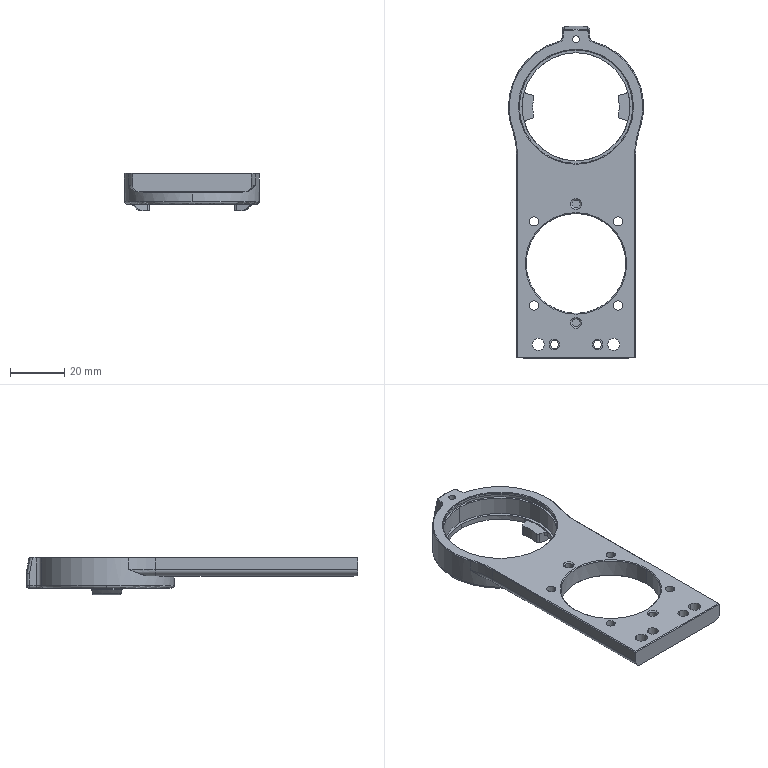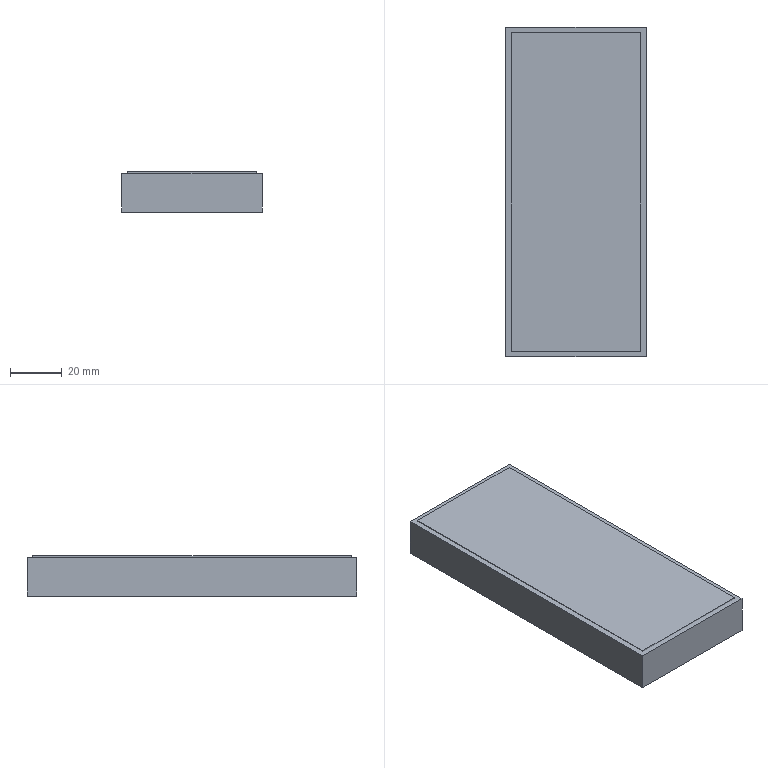CAM job | NX | 3-axis milling, drilling | part box 50 x 122.9 x 14 mm | stock box 54 x 126.9 x 15.5 mm
Tools:
number,name,description,diameter,corner_radius,flute_length,length,flutes
19,D80,Milling Tool-5 Parameters,80.0,0.0,50.0,75.0,2
1,D6A45,Milling Tool-5 Parameters,6.0,0.0,50.0,75.0,2
15,D10,Milling Tool-5 Parameters,10.0,0.0,50.0,75.0,2
14,D10JING,Milling Tool-5 Parameters,10.0,0.0,50.0,75.0,2
8,4.5ZT,Drilling Tool,4.5,0.0,35.0,50.0,2
16,3.0ZT,Drilling Tool,3.0,0.0,35.0,50.0,2
7,3.4ZT,Drilling Tool,3.4,0.0,35.0,50.0,2
2,2.5ZT,Drilling Tool,2.5,0.0,35.0,50.0,2
17,D2,Milling Tool-5 Parameters,2.0,0.0,50.0,75.0,2
18,D3R0.5,Milling Tool-5 Parameters,3.0,0.5,50.0,75.0,2
21,T6H4D1.5,Milling Tool-T Cutter,6.0,,1.5,25.0,4
11,D4,Milling Tool-5 Parameters,4.0,0.0,50.0,75.0,2
Operations:
program,operation,operation_type,tool,method,geometry_group,spindle_rpm,surface_speed,feed_per_tooth,feed_cut,feed_plunge,cut_length_mm,path_length_mm,cut_time_min,machine_time_min
1,FLOOR_WALL,VolumeBased25DMillingOperation,D80,METHOD,A,5000.0,1256.0,0.12,1200.0,100.0,218.9,272.9,0.1824,0.1878
1,ZLEVEL_PROFILE,ZLevelMilling,D10,METHOD,A,9500.0,298.0,0.1842,3500.0,1000.0,6306.798,6377.798,1.833,1.84
1,HOLE_MILLING,CylinderMilling,D10,METHOD,A,9500.0,0.0,0.0,2500.0,1000.0,781.06,847.56,0.3148,0.3214
1,HOLE_MILLING_COPY,CylinderMilling,D10,METHOD,A,9500.0,0.0,0.0,2500.0,1000.0,974.372,1043.872,0.3921,0.3991
1,ZLEVEL_PROFILE_COPY,ZLevelMilling,D10JING,METHOD,A,9500.0,298.0,0.0789,1500.0,1000.0,377.945,462.945,0.2615,0.27
1,HOLE_MILLING_COPY_COPY,CylinderMilling,D10JING,METHOD,A,9500.0,0.0,0.1053,2000.0,1000.0,1146.72,1215.745,0.5829,0.5898
1,HOLE_MILLING_COPY_COPY_COPY,CylinderMilling,D10JING,METHOD,A,9500.0,0.0,0.1053,2000.0,1000.0,287.94,348.44,0.1529,0.159
1,SPOT_DRILLING,Operation,D6A45,METHOD,A,9500.0,179.0,0.0132,250.0,0.0,52.0,415.591,0.208,0.2444
1,DRILLING,Operation,4.5ZT,METHOD,A,2500.0,35.0,0.04,200.0,0.0,18.904,128.968,0.0945,0.1055
1,DRILLING_COPY,Operation,3.0ZT,METHOD,A,2500.0,35.0,0.04,200.0,0.0,24.803,128.884,0.124,0.1344
1,DRILLING_COPY_COPY,Operation,3.4ZT,METHOD,A,2500.0,35.0,0.04,200.0,0.0,50.086,262.943,0.2504,0.2717
1,DRILLING_COPY_COPY_COPY,Operation,2.5ZT,METHOD,A,2500.0,19.0,0.02,100.0,0.0,16.751,93.502,0.1675,0.1752
1,HOLE_MILLING_1,CylinderMilling,D2,METHOD,A,9500.0,59.0,0.0553,1050.0,100.0,639.065,964.378,0.6086,0.6412
1,ZLEVEL_PROFILE_1,ZLevelMilling,D3R0.5,METHOD,A,9500.0,89.0,0.1316,2500.0,1000.0,1324.38,1546.793,0.5389,0.5611
1,ZLEVEL_PROFILE_COPY_1,ZLevelMilling,D3R0.5,METHOD,A,9500.0,298.0,0.1842,3500.0,1000.0,345.377,683.941,0.144,0.1779
1,PLANAR_PROFILE,PlanarMilling,D6A45,METHOD,A,9500.0,179.0,0.0789,1500.0,100.0,715.283,1785.284,0.4769,0.5839
1,PLANAR_MILL,PlanarMilling,T6H4D1.5,METHOD,A,9500.0,179.0,0.0329,1250.0,100.0,366.114,425.114,0.2929,0.2988
2,FLOOR_WALL_COPY,VolumeBased25DMillingOperation,D80,METHOD,B,5000.0,1256.0,0.12,1200.0,100.0,437.8,756.9,0.3648,0.3967
2,FLOOR_WALL_COPY_COPY,VolumeBased25DMillingOperation,D80,METHOD,B,5000.0,1256.0,0.12,1200.0,100.0,218.9,272.9,0.1824,0.1878
2,FLOOR_WALL_1,VolumeBased25DMillingOperation,D10,METHOD,B,9500.0,298.0,0.1316,2500.0,1000.0,6466.524,6677.464,2.786,2.807
2,FLOOR_WALL_1_COPY,VolumeBased25DMillingOperation,D10,METHOD,B,9500.0,298.0,0.1316,2500.0,1000.0,1917.348,2034.197,0.855,0.8667
2,ZLEVEL_PROFILE_COPY_2,ZLevelMilling,D10,METHOD,B,9500.0,298.0,0.1053,2000.0,1000.0,461.743,836.252,0.2434,0.2808
2,FLOOR_WALL_1_COPY_1,VolumeBased25DMillingOperation,D4,METHOD,B,9500.0,119.0,0.1053,2000.0,1000.0,4963.452,5168.629,2.844,2.864
2,FLOOR_WALL_1_COPY_1_COPY,VolumeBased25DMillingOperation,D4,METHOD,B,9500.0,119.0,0.1053,2000.0,1000.0,1096.978,1373.241,0.8775,0.9052
2,HOLE_MILLING_2,CylinderMilling,D4,METHOD,B,9500.0,119.0,0.0658,1250.0,100.0,212.223,394.023,0.1698,0.188
2,FLOOR_WALL_1_COPY_1_COPY_COPY,VolumeBased25DMillingOperation,D4,METHOD,B,9500.0,119.0,0.0632,1200.0,1000.0,2509.889,3688.856,2.104,2.221
2,ZLEVEL_PROFILE_1_COPY,ZLevelMilling,D3R0.5,METHOD,B,9500.0,89.0,0.1316,2500.0,1000.0,5074.066,5329.071,2.039,2.064
2,ZLEVEL_PROFILE_1_COPY_COPY,ZLevelMilling,D3R0.5,METHOD,B,9500.0,89.0,0.1316,2500.0,1000.0,3843.192,4206.281,1.551,1.587
2,ZLEVEL_PROFILE_1_COPY_COPY_1,ZLevelMilling,D3R0.5,METHOD,B,9500.0,89.0,0.1316,2500.0,1000.0,2779.932,3021.218,1.122,1.146
2,ZLEVEL_PROFILE_1_COPY_COPY_1_COPY,ZLevelMilling,D3R0.5,METHOD,B,9500.0,89.0,0.1316,2500.0,1000.0,2517.762,2667.223,1.015,1.03
2,ZLEVEL_PROFILE_1_COPY_COPY_1_COPY_COPY,ZLevelMilling,D3R0.5,METHOD,B,9500.0,89.0,0.1316,2500.0,1000.0,7627.648,7820.681,3.057,3.076
2,ZLEVEL_PROFILE_COPY_2_COPY,ZLevelMilling,D2,METHOD,B,9500.0,59.0,0.0526,1000.0,1000.0,548.153,1099.402,0.5482,0.6033
2,PLANAR_MILL_1,PlanarMilling,D6A45,METHOD,B,9500.0,179.0,0.0658,1250.0,100.0,323.199,1202.471,0.2586,0.3465
2,PLANAR_MILL_1_COPY,PlanarMilling,D6A45,METHOD,B,9500.0,179.0,0.0658,1250.0,100.0,120.878,337.675,0.0967,0.1184
2,PLANAR_MILL_1_COPY_COPY,PlanarMilling,D6A45,METHOD,B,9500.0,179.0,0.0658,1250.0,100.0,102.569,251.551,0.0821,0.097
2,PLANAR_MILL_1_COPY_COPY_COPY,PlanarMilling,D6A45,METHOD,B,9500.0,179.0,0.0658,1250.0,100.0,46.236,202.614,0.037,0.0526
3,HOLE_MILLING_COPY_COPY_COPY_1,CylinderMilling,D10JING,METHOD,A,9500.0,0.0,0.1053,2000.0,1000.0,1145.152,1214.178,0.5817,0.5886